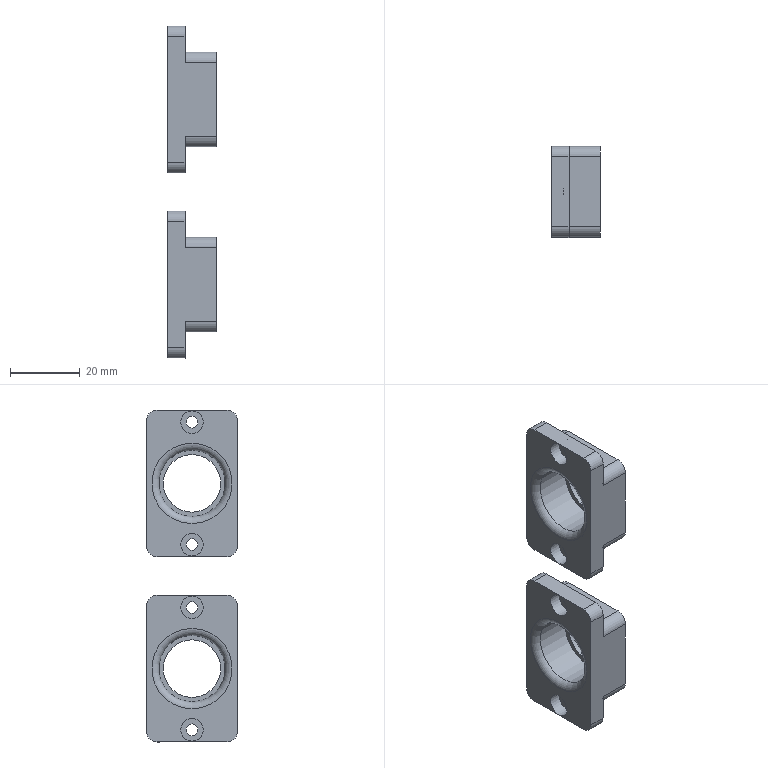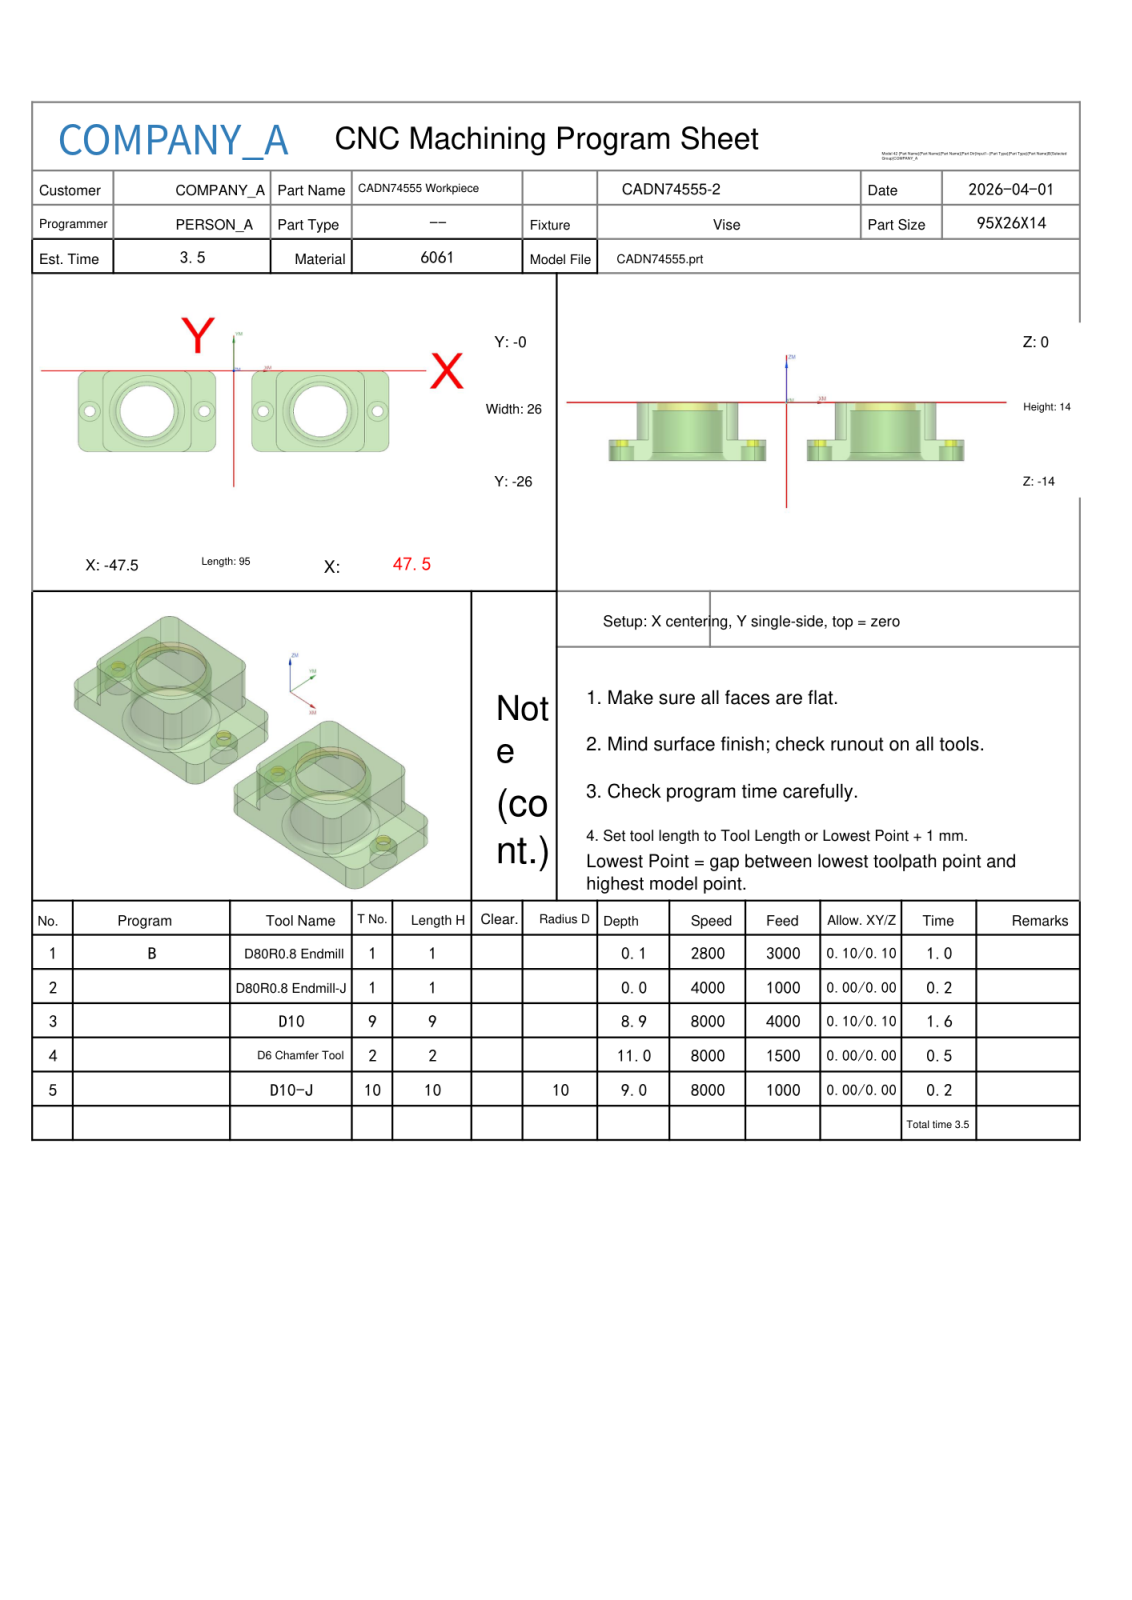NC program | NX | posted by the shop | part box 14 x 26 x 95 mm
Whole program:
%
O0001
(Machine time: 4.41 MIN)
(===Total Tool:4===)
(T1=D80R0.8 Endmill D=80.  R=0.8  D-  H01 Z=0.    )
(T9=D10     D=10.  R=0.   D-  H09 Z=-8.9  )
(T2=D6 Chamfer tool   D=6.   R=0.   D-  H02 Z=-11.  )
(T10=D10-J  D=10.  R=0.   D10 H10 Z=-9.   )
G80 G90 G17 G49 G40
G91 G28 Z0
M01
N1 T01 M06
(D80R0.8 Endmill  D=80. R=0.8 H=01 ce=0.10 di=0.10)
G00 G90 G54 X-99.597 Y-13.002 M03 S2800
G43 H01 Z20.
M08
Z7.009
G01 Z5.009 F3000.
X-87.597
X87.597 Y-12.998
X99.597
Z7.009
G00 X-99.597 Y-13.002
Z6.518
G01 Z4.518
X-87.597
X87.597 Y-12.998
X99.597
Z6.518
G00 X-99.597 Y-13.002
Z6.027
G01 Z4.027
X-87.597
X87.597 Y-12.998
X99.597
Z6.027
G00 X-99.597 Y-13.002
Z5.536
G01 Z3.536
X-87.597
X87.597 Y-12.998
X99.597
Z5.536
G00 Z20.
X-99.597 Y-13.002
Z5.045
G01 Z3.045
X-87.597
X87.597 Y-12.998
X99.597
Z5.045
G00 Z20.
X-99.597 Y-13.002
Z4.555
G01 Z2.555
X-87.597
X87.597 Y-12.998
X99.597
Z4.555
G00 Z20.
X-99.597 Y-13.002
Z4.064
G01 Z2.064
X-87.597
X87.597 Y-12.998
X99.597
Z4.064
G00 Z20.
X-99.597 Y-13.002
Z3.573
G01 Z1.573
X-87.597
X87.597 Y-12.998
X99.597
Z3.573
G00 Z20.
X-99.597 Y-13.002
Z3.082
G01 Z1.082
X-87.597
X87.597 Y-12.998
X99.597
Z3.082
G00 Z20.
X-99.597 Y-13.002
Z2.591
G01 Z.591
X-87.597
X87.597 Y-12.998
X99.597
Z2.591
G00 Z20.
X-99.597 Y-13.002
Z2.1
G01 Z.1
X-87.597
X87.597 Y-12.998
X99.597
Z2.1
G00 Z20.
G91 G28 Z0.0
M05
M09
G91 G28 Z0.0
M01
N2 T01 M06
(D80R0.8 Endmill-J  D=80. R=0.8 H=01 ce=0.00 di=0.00)
G00 G90 G54 X-99.499 Y-13. M03 S4000
G43 H01 Z20.
M08
Z2.
G01 Z0.0 F1000.
X-87.499
X87.499
X99.499
Z2.
G00 Z20.
G91 G28 Z0.0
M05
M09
G91 G28 Z0.0
M01
N3 T09 M06
(D10  D=10. R=0. H=09 ce=0.10 di=0.10)
G00 G90 G54 X-55.5 Y-13. M03 S8000
G43 H09 Z15.5
M08
Z.907
G01 Z-.593 F4000.
X-52.4
Y-3.
G02 X-44.5 Y4.9 I7.9 J0.0
G01 X-38.789
G03 X-45.1 Y-3. I1.789 J-7.9
G01 Y-23.
G03 X-38.789 Y-30.9 I8.1 J0.0
G01 X-44.5
G02 X-52.4 Y-23. I0.0 J7.9
G01 Y-13.
Y-12.5
X-55.5
Z.907
G00 Y-13.
Z.313
G01 Z-1.187
X-52.4
Y-3.
G02 X-44.5 Y4.9 I7.9 J0.0
G01 X-38.789
G03 X-45.1 Y-3. I1.789 J-7.9
G01 Y-23.
G03 X-38.789 Y-30.9 I8.1 J0.0
G01 X-44.5
G02 X-52.4 Y-23. I0.0 J7.9
G01 Y-13.
Y-12.5
X-55.5
Z.313
G00 Y-13.
Z-.28
G01 Z-1.78
X-52.4
Y-3.
G02 X-44.5 Y4.9 I7.9 J0.0
G01 X-38.789
G03 X-45.1 Y-3. I1.789 J-7.9
G01 Y-23.
G03 X-38.789 Y-30.9 I8.1 J0.0
G01 X-44.5
G02 X-52.4 Y-23. I0.0 J7.9
G01 Y-13.
Y-12.5
X-55.5
Z-.28
G00 Y-13.
Z-.873
G01 Z-2.373
X-52.4
Y-3.
G02 X-44.5 Y4.9 I7.9 J0.0
G01 X-38.789
G03 X-45.1 Y-3. I1.789 J-7.9
G01 Y-23.
G03 X-38.789 Y-30.9 I8.1 J0.0
G01 X-44.5
G02 X-52.4 Y-23. I0.0 J7.9
G01 Y-13.
Y-12.5
X-55.5
Z-.873
G00 Y-13.
Z-1.467
G01 Z-2.967
X-52.4
Y-3.
G02 X-44.5 Y4.9 I7.9 J0.0
G01 X-38.789
G03 X-45.1 Y-3. I1.789 J-7.9
G01 Y-23.
G03 X-38.789 Y-30.9 I8.1 J0.0
G01 X-44.5
G02 X-52.4 Y-23. I0.0 J7.9
G01 Y-13.
Y-12.5
X-55.5
Z-1.467
G00 Y-13.
Z-2.06
G01 Z-3.56
X-52.4
Y-3.
G02 X-44.5 Y4.9 I7.9 J0.0
G01 X-38.789
G03 X-45.1 Y-3. I1.789 J-7.9
G01 Y-23.
G03 X-38.789 Y-30.9 I8.1 J0.0
G01 X-44.5
G02 X-52.4 Y-23. I0.0 J7.9
G01 Y-13.
Y-12.5
X-55.5
Z-2.06
G00 Y-13.
Z-2.653
G01 Z-4.153
X-52.4
Y-3.
G02 X-44.5 Y4.9 I7.9 J0.0
G01 X-38.789
G03 X-45.1 Y-3. I1.789 J-7.9
G01 Y-23.
G03 X-38.789 Y-30.9 I8.1 J0.0
G01 X-44.5
G02 X-52.4 Y-23. I0.0 J7.9
G01 Y-13.
Y-12.5
X-55.5
Z-2.653
G00 Y-13.
Z-3.247
G01 Z-4.747
X-52.4
Y-3.
G02 X-44.5 Y4.9 I7.9 J0.0
G01 X-38.789
G03 X-45.1 Y-3. I1.789 J-7.9
G01 Y-23.
G03 X-38.789 Y-30.9 I8.1 J0.0
G01 X-44.5
G02 X-52.4 Y-23. I0.0 J7.9
G01 Y-13.
Y-12.5
X-55.5
Z-3.247
G00 Y-13.
Z-3.84
G01 Z-5.34
X-52.4
Y-3.
G02 X-44.5 Y4.9 I7.9 J0.0
G01 X-38.789
G03 X-45.1 Y-3. I1.789 J-7.9
G01 Y-23.
G03 X-38.789 Y-30.9 I8.1 J0.0
G01 X-44.5
G02 X-52.4 Y-23. I0.0 J7.9
G01 Y-13.
Y-12.5
X-55.5
Z-3.84
G00 Y-13.
Z-4.433
G01 Z-5.933
X-52.4
Y-3.
G02 X-44.5 Y4.9 I7.9 J0.0
G01 X-38.789
G03 X-45.1 Y-3. I1.789 J-7.9
G01 Y-23.
G03 X-38.789 Y-30.9 I8.1 J0.0
G01 X-44.5
G02 X-52.4 Y-23. I0.0 J7.9
G01 Y-13.
Y-12.5
X-55.5
Z-4.433
G00 Y-13.
Z-5.027
G01 Z-6.527
X-52.4
Y-3.
G02 X-44.5 Y4.9 I7.9 J0.0
G01 X-38.789
G03 X-45.1 Y-3. I1.789 J-7.9
G01 Y-23.
G03 X-38.789 Y-30.9 I8.1 J0.0
G01 X-44.5
G02 X-52.4 Y-23. I0.0 J7.9
G01 Y-13.
Y-12.5
X-55.5
Z-5.027
G00 Y-13.
Z-5.62
G01 Z-7.12
X-52.4
Y-3.
G02 X-44.5 Y4.9 I7.9 J0.0
G01 X-38.789
G03 X-45.1 Y-3. I1.789 J-7.9
G01 Y-23.
G03 X-38.789 Y-30.9 I8.1 J0.0
G01 X-44.5
G02 X-52.4 Y-23. I0.0 J7.9
G01 Y-13.
Y-12.5
X-55.5
Z-5.62
G00 Y-13.
Z-6.213
G01 Z-7.713
X-52.4
Y-3.
G02 X-44.5 Y4.9 I7.9 J0.0
G01 X-38.789
G03 X-45.1 Y-3. I1.789 J-7.9
G01 Y-23.
G03 X-38.789 Y-30.9 I8.1 J0.0
G01 X-44.5
G02 X-52.4 Y-23. I0.0 J7.9
G01 Y-13.
Y-12.5
X-55.5
Z-6.213
G00 Y-13.
Z-6.807
G01 Z-8.307
X-52.4
Y-3.
G02 X-44.5 Y4.9 I7.9 J0.0
G01 X-38.789
G03 X-45.1 Y-3. I1.789 J-7.9
G01 Y-23.
G03 X-38.789 Y-30.9 I8.1 J0.0
G01 X-44.5
G02 X-52.4 Y-23. I0.0 J7.9
G01 Y-13.
Y-12.5
X-55.5
Z-6.807
G00 Y-13.
Z-7.4
G01 Z-8.9
X-52.4
Y-3.
G02 X-44.5 Y4.9 I7.9 J0.0
G01 X-38.789
G03 X-45.1 Y-3. I1.789 J-7.9
G01 Y-23.
G03 X-38.789 Y-30.9 I8.1 J0.0
G01 X-44.5
G02 X-52.4 Y-23. I0.0 J7.9
G01 Y-13.
Y-12.5
X-55.5
Z-7.4
G00 Z15.5
X0.0 Y-33.269
Z.907
G01 Z-.593
Y-30.169
X-5.182
X-5.201 Y-30.178
G02 X-8.5 Y-30.9 I-3.299 J7.178
G01 X-14.211
G03 X-7.9 Y-23. I-1.789 J7.9
G01 Y-3.
G03 X-14.211 Y4.9 I-8.1 J0.0
G01 X-8.5
G02 X-5.181 Y4.169 I0.0 J-7.9
G01 X5.201 Y4.178
G02 X8.5 Y4.9 I3.299 J-7.178
G01 X14.211
G03 X7.9 Y-3. I1.789 J-7.9
G01 Y-23.
G03 X14.211 Y-30.9 I8.1 J0.0
G01 X8.5
G02 X5.181 Y-30.169 I0.0 J7.9
G01 X3.222
G02 X2.273 Y-29.486 I0.0 J1.
G01 X.141 Y-23.096
G03 X-.23 Y-22.596 I-.948 J-.317
G02 X-.4 Y-22.271 I.23 J.327
G01 Y-3.729
G02 X0.0 Y-3.331 I.4 J-.001
X.4 Y-3.729 I0.0 J-.4
G01 Y-22.271
G02 X.001 Y-22.669 I-.4 J.001
G01 X-.001
G02 X-.379 Y-22.397 I.001 J.4
G01 X-3.223 Y-23.352
Z.907
G00 X0.0 Y-33.269
Z.313
G01 Z-1.187
Y-30.169
X-5.182
X-5.201 Y-30.178
G02 X-8.5 Y-30.9 I-3.299 J7.178
G01 X-14.211
G03 X-7.9 Y-23. I-1.789 J7.9
G01 Y-3.
G03 X-14.211 Y4.9 I-8.1 J0.0
G01 X-8.5
G02 X-5.181 Y4.169 I0.0 J-7.9
G01 X5.201 Y4.178
G02 X8.5 Y4.9 I3.299 J-7.178
G01 X14.211
G03 X7.9 Y-3. I1.789 J-7.9
G01 Y-23.
G03 X14.211 Y-30.9 I8.1 J0.0
G01 X8.5
G02 X5.181 Y-30.169 I0.0 J7.9
G01 X3.222
G02 X2.273 Y-29.486 I0.0 J1.
G01 X.141 Y-23.096
G03 X-.23 Y-22.596 I-.948 J-.317
G02 X-.4 Y-22.271 I.23 J.327
G01 Y-3.729
G02 X0.0 Y-3.331 I.4 J-.001
X.4 Y-3.729 I0.0 J-.4
G01 Y-22.271
G02 X.001 Y-22.669 I-.4 J.001
G01 X-.001
G02 X-.379 Y-22.397 I.001 J.4
G01 X-3.223 Y-23.352
Z.313
G00 X0.0 Y-33.269
Z-.28
G01 Z-1.78
Y-30.169
X-5.182
X-5.201 Y-30.178
G02 X-8.5 Y-30.9 I-3.299 J7.178
G01 X-14.211
G03 X-7.9 Y-23. I-1.789 J7.9
G01 Y-3.
G03 X-14.211 Y4.9 I-8.1 J0.0
G01 X-8.5
G02 X-5.181 Y4.169 I0.0 J-7.9
G01 X5.201 Y4.178
G02 X8.5 Y4.9 I3.299 J-7.178
G01 X14.211
G03 X7.9 Y-3. I1.789 J-7.9
G01 Y-23.
G03 X14.211 Y-30.9 I8.1 J0.0
G01 X8.5
G02 X5.181 Y-30.169 I0.0 J7.9
G01 X3.222
G02 X2.273 Y-29.486 I0.0 J1.
G01 X.141 Y-23.096
G03 X-.23 Y-22.596 I-.948 J-.317
G02 X-.4 Y-22.271 I.23 J.327
G01 Y-3.729
G02 X0.0 Y-3.331 I.4 J-.001
X.4 Y-3.729 I0.0 J-.4
G01 Y-22.271
G02 X.001 Y-22.669 I-.4 J.001
G01 X-.001
G02 X-.379 Y-22.397 I.001 J.4
G01 X-3.223 Y-23.352
Z-.28
G00 X0.0 Y-33.269
Z-.873
G01 Z-2.373
Y-30.169
X-5.182
X-5.201 Y-30.178
G02 X-8.5 Y-30.9 I-3.299 J7.178
G01 X-14.211
G03 X-7.9 Y-23. I-1.789 J7.9
G01 Y-3.
G03 X-14.211 Y4.9 I-8.1 J0.0
G01 X-8.5
G02 X-5.181 Y4.169 I0.0 J-7.9
G01 X5.201 Y4.178
G02 X8.5 Y4.9 I3.299 J-7.178
G01 X14.211
G03 X7.9 Y-3. I1.789 J-7.9
G01 Y-23.
G03 X14.211 Y-30.9 I8.1 J0.0
G01 X8.5
G02 X5.181 Y-30.169 I0.0 J7.9
G01 X3.222
G02 X2.273 Y-29.486 I0.0 J1.
G01 X.141 Y-23.096
G03 X-.23 Y-22.596 I-.948 J-.317
G02 X-.4 Y-22.271 I.23 J.327
G01 Y-3.729
G02 X0.0 Y-3.331 I.4 J-.001
X.4 Y-3.729 I0.0 J-.4
G01 Y-22.271
G02 X.001 Y-22.669 I-.4 J.001
G01 X-.001
G02 X-.379 Y-22.397 I.001 J.4
G01 X-3.223 Y-23.352
Z-.873
G00 X0.0 Y-33.269
Z-1.467
G01 Z-2.967
Y-30.169
X-5.182
X-5.201 Y-30.178
G02 X-8.5 Y-30.9 I-3.299 J7.178
G01 X-14.211
G03 X-7.9 Y-23. I-1.789 J7.9
G01 Y-3.
G03 X-14.211 Y4.9 I-8.1 J0.0
G01 X-8.5
G02 X-5.181 Y4.169 I0.0 J-7.9
G01 X5.201 Y4.178
G02 X8.5 Y4.9 I3.299 J-7.178
G01 X14.211
G03 X7.9 Y-3. I1.789 J-7.9
G01 Y-23.
G03 X14.211 Y-30.9 I8.1 J0.0
G01 X8.5
G02 X5.181 Y-30.169 I0.0 J7.9
G01 X3.222
G02 X2.273 Y-29.486 I0.0 J1.
G01 X.141 Y-23.096
G03 X-.23 Y-22.596 I-.948 J-.317
G02 X-.4 Y-22.271 I.23 J.327
G01 Y-3.729
G02 X0.0 Y-3.331 I.4 J-.001
X.4 Y-3.729 I0.0 J-.4
G01 Y-22.271
G02 X.001 Y-22.669 I-.4 J.001
G01 X-.001
G02 X-.379 Y-22.397 I.001 J.4
G01 X-3.223 Y-23.352
Z-1.467
G00 X0.0 Y-33.269
Z-2.06
G01 Z-3.56
Y-30.169
X-5.182
X-5.201 Y-30.178
G02 X-8.5 Y-30.9 I-3.299 J7.178
G01 X-14.211
G03 X-7.9 Y-23. I-1.789 J7.9
G01 Y-3.
G03 X-14.211 Y4.9 I-8.1 J0.0
G01 X-8.5
G02 X-5.181 Y4.169 I0.0 J-7.9
G01 X5.201 Y4.178
G02 X8.5 Y4.9 I3.299 J-7.178
G01 X14.211
G03 X7.9 Y-3. I1.789 J-7.9
G01 Y-23.
G03 X14.211 Y-30.9 I8.1 J0.0
G01 X8.5
G02 X5.181 Y-30.169 I0.0 J7.9
G01 X3.222
G02 X2.273 Y-29.486 I0.0 J1.
G01 X.141 Y-23.096
G03 X-.23 Y-22.596 I-.948 J-.317
G02 X-.4 Y-22.271 I.23 J.327
G01 Y-3.729
G02 X0.0 Y-3.331 I.4 J-.001
X.4 Y-3.729 I0.0 J-.4
G01 Y-22.271
G02 X.001 Y-22.669 I-.4 J.001
G01 X-.001
G02 X-.379 Y-22.397 I.001 J.4
G01 X-3.223 Y-23.352
Z-2.06
G00 X0.0 Y-33.269
Z-2.653
G01 Z-4.153
Y-30.169
X-5.182
X-5.201 Y-30.178
G02 X-8.5 Y-30.9 I-3.299 J7.178
G01 X-14.211
G03 X-7.9 Y-23. I-1.789 J7.9
G01 Y-3.
G03 X-14.211 Y4.9 I-8.1 J0.0
G01 X-8.5
G02 X-5.181 Y4.169 I0.0 J-7.9
G01 X5.201 Y4.178
G02 X8.5 Y4.9 I3.299 J-7.178
G01 X14.211
G03 X7.9 Y-3. I1.789 J-7.9
G01 Y-23.
G03 X14.211 Y-30.9 I8.1 J0.0
G01 X8.5
G02 X5.181 Y-30.169 I0.0 J7.9
G01 X3.222
G02 X2.273 Y-29.486 I0.0 J1.
G01 X.141 Y-23.096
G03 X-.23 Y-22.596 I-.948 J-.317
G02 X-.4 Y-22.271 I.23 J.327
G01 Y-3.729
G02 X0.0 Y-3.331 I.4 J-.001
X.4 Y-3.729 I0.0 J-.4
G01 Y-22.271
G02 X.001 Y-22.669 I-.4 J.001
G01 X-.001
G02 X-.379 Y-22.397 I.001 J.4
G01 X-3.223 Y-23.352
Z-2.653
G00 X0.0 Y-33.269
Z-3.247
G01 Z-4.747
Y-30.169
X-5.182
X-5.201 Y-30.178
G02 X-8.5 Y-30.9 I-3.299 J7.178
G01 X-14.211
G03 X-7.9 Y-23. I-1.789 J7.9
G01 Y-3.
G03 X-14.211 Y4.9 I-8.1 J0.0
G01 X-8.5
G02 X-5.181 Y4.169 I0.0 J-7.9
G01 X5.201 Y4.178
G02 X8.5 Y4.9 I3.299 J-7.178
G01 X14.211
G03 X7.9 Y-3. I1.789 J-7.9
G01 Y-23.
G03 X14.211 Y-30.9 I8.1 J0.0
G01 X8.5
G02 X5.181 Y-30.169 I0.0 J7.9
G01 X3.222
G02 X2.273 Y-29.486 I0.0 J1.
G01 X.141 Y-23.096
G03 X-.23 Y-22.596 I-.948 J-.317
G02 X-.4 Y-22.271 I.23 J.327
G01 Y-3.729
G02 X0.0 Y-3.331 I.4 J-.001
X.4 Y-3.729 I0.0 J-.4
G01 Y-22.271
G02 X.001 Y-22.669 I-.4 J.001
G01 X-.001
G02 X-.379 Y-22.397 I.001 J.4
G01 X-3.223 Y-23.352
Z-3.247
G00 X0.0 Y-33.269
Z-3.84
G01 Z-5.34
Y-30.169
X-5.182
X-5.201 Y-30.178
G02 X-8.5 Y-30.9 I-3.299 J7.178
G01 X-14.211
G03 X-7.9 Y-23. I-1.789 J7.9
G01 Y-3.
G03 X-14.211 Y4.9 I-8.1 J0.0
G01 X-8.5
G02 X-5.181 Y4.169 I0.0 J-7.9
G01 X5.201 Y4.178
G02 X8.5 Y4.9 I3.299 J-7.178
G01 X14.211
G03 X7.9 Y-3. I1.789 J-7.9
G01 Y-23.
G03 X14.211 Y-30.9 I8.1 J0.0
G01 X8.5
G02 X5.181 Y-30.169 I0.0 J7.9
G01 X3.222
G02 X2.273 Y-29.486 I0.0 J1.
G01 X.141 Y-23.096
G03 X-.23 Y-22.596 I-.948 J-.317
G02 X-.4 Y-22.271 I.23 J.327
G01 Y-3.729
G02 X0.0 Y-3.331 I.4 J-.001
X.4 Y-3.729 I0.0 J-.4
G01 Y-22.271
G02 X.001 Y-22.669 I-.4 J.001
G01 X-.001
G02 X-.379 Y-22.397 I.001 J.4
G01 X-3.223 Y-23.352
Z-3.84
G00 X0.0 Y-33.269
Z-4.433
G01 Z-5.933
Y-30.169
X-5.182
X-5.201 Y-30.178
G02 X-8.5 Y-30.9 I-3.299 J7.178
G01 X-14.211
G03 X-7.9 Y-23. I-1.789 J7.9
G01 Y-3.
G03 X-14.211 Y4.9 I-8.1 J0.0
G01 X-8.5
G02 X-5.181 Y4.169 I0.0 J-7.9
G01 X5.201 Y4.178
G02 X8.5 Y4.9 I3.299 J-7.178
G01 X14.211
G03 X7.9 Y-3. I1.789 J-7.9
G01 Y-23.
G03 X14.211 Y-30.9 I8.1 J0.0
G01 X8.5
G02 X5.181 Y-30.169 I0.0 J7.9
G01 X3.222
G02 X2.273 Y-29.486 I0.0 J1.
G01 X.141 Y-23.096
G03 X-.23 Y-22.596 I-.948 J-.317
G02 X-.4 Y-22.271 I.23 J.327
G01 Y-3.729
G02 X0.0 Y-3.331 I.4 J-.001
X.4 Y-3.729 I0.0 J-.4
G01 Y-22.271
G02 X.001 Y-22.669 I-.4 J.001
G01 X-.001
G02 X-.379 Y-22.397 I.001 J.4
G01 X-3.223 Y-23.352
Z-4.433
G00 X0.0 Y-33.269
Z-5.027
G01 Z-6.527
Y-30.169
X-5.182
X-5.201 Y-30.178
G02 X-8.5 Y-30.9 I-3.299 J7.178
G01 X-14.211
G03 X-7.9 Y-23. I-1.789 J7.9
G01 Y-3.
G03 X-14.211 Y4.9 I-8.1 J0.0
G01 X-8.5
G02 X-5.181 Y4.169 I0.0 J-7.9
G01 X5.201 Y4.178
G02 X8.5 Y4.9 I3.299 J-7.178
G01 X14.211
G03 X7.9 Y-3. I1.789 J-7.9
G01 Y-23.
G03 X14.211 Y-30.9 I8.1 J0.0
G01 X8.5
G02 X5.181 Y-30.169 I0.0 J7.9
G01 X3.222
G02 X2.273 Y-29.486 I0.0 J1.
G01 X.141 Y-23.096
G03 X-.23 Y-22.596 I-.948 J-.317
G02 X-.4 Y-22.271 I.23 J.327
G01 Y-3.729
G02 X0.0 Y-3.331 I.4 J-.001
X.4 Y-3.729 I0.0 J-.4
G01 Y-22.271
G02 X.001 Y-22.669 I-.4 J.001
G01 X-.001
G02 X-.379 Y-22.397 I.001 J.4
G01 X-3.223 Y-23.352
Z-5.027
G00 X0.0 Y-33.269
Z-5.62
G01 Z-7.12
Y-30.169
X-5.182
X-5.201 Y-30.178
G02 X-8.5 Y-30.9 I-3.299 J7.178
G01 X-14.211
G03 X-7.9 Y-23. I-1.789 J7.9
G01 Y-3.
G03 X-14.211 Y4.9 I-8.1 J0.0
G01 X-8.5
G02 X-5.181 Y4.169 I0.0 J-7.9
G01 X5.201 Y4.178
G02 X8.5 Y4.9 I3.299 J-7.178
G01 X14.211
G03 X7.9 Y-3. I1.789 J-7.9
G01 Y-23.
G03 X14.211 Y-30.9 I8.1 J0.0
G01 X8.5
G02 X5.181 Y-30.169 I0.0 J7.9
G01 X3.222
G02 X2.273 Y-29.486 I0.0 J1.
G01 X.141 Y-23.096
G03 X-.23 Y-22.596 I-.948 J-.317
G02 X-.4 Y-22.271 I.23 J.327
G01 Y-3.729
G02 X0.0 Y-3.331 I.4 J-.001
X.4 Y-3.729 I0.0 J-.4
G01 Y-22.271
G02 X.001 Y-22.669 I-.4 J.001
G01 X-.001
G02 X-.379 Y-22.397 I.001 J.4
G01 X-3.223 Y-23.352
Z-5.62
G00 X0.0 Y-33.269
Z-6.213
G01 Z-7.713
Y-30.169
X-5.182
X-5.201 Y-30.178
G02 X-8.5 Y-30.9 I-3.299 J7.178
G01 X-14.211
G03 X-7.9 Y-23. I-1.789 J7.9
G01 Y-3.
G03 X-14.211 Y4.9 I-8.1 J0.0
G01 X-8.5
G02 X-5.181 Y4.169 I0.0 J-7.9
G01 X5.201 Y4.178
G02 X8.5 Y4.9 I3.299 J-7.178
G01 X14.211
G03 X7.9 Y-3. I1.789 J-7.9
G01 Y-23.
G03 X14.211 Y-30.9 I8.1 J0.0
G01 X8.5
G02 X5.181 Y-30.169 I0.0 J7.9
G01 X3.222
G02 X2.273 Y-29.486 I0.0 J1.
G01 X.141 Y-23.096
G03 X-.23 Y-22.596 I-.948 J-.317
G02 X-.4 Y-22.271 I.23 J.327
G01 Y-3.729
G02 X0.0 Y-3.331 I.4 J-.001
X.4 Y-3.729 I0.0 J-.4
G01 Y-22.271
G02 X.001 Y-22.669 I-.4 J.001
G01 X-.001
G02 X-.379 Y-22.397 I.001 J.4
G01 X-3.223 Y-23.352
Z-6.213
G00 X0.0 Y-33.269
Z-6.807
G01 Z-8.307
Y-30.169
X-5.182
X-5.201 Y-30.178
G02 X-8.5 Y-30.9 I-3.299 J7.178
G01 X-14.211
G03 X-7.9 Y-23. I-1.789 J7.9
G01 Y-3.
G03 X-14.211 Y4.9 I-8.1 J0.0
G01 X-8.5
G02 X-5.181 Y4.169 I0.0 J-7.9
G01 X5.201 Y4.178
G02 X8.5 Y4.9 I3.299 J-7.178
G01 X14.211
G03 X7.9 Y-3. I1.789 J-7.9
G01 Y-23.
G03 X14.211 Y-30.9 I8.1 J0.0
G01 X8.5
G02 X5.181 Y-30.169 I0.0 J7.9
G01 X3.222
G02 X2.273 Y-29.486 I0.0 J1.
G01 X.141 Y-23.096
G03 X-.23 Y-22.596 I-.948 J-.317
G02 X-.4 Y-22.271 I.23 J.327
G01 Y-3.729
G02 X0.0 Y-3.331 I.4 J-.001
X.4 Y-3.729 I0.0 J-.4
G01 Y-22.271
G02 X.001 Y-22.669 I-.4 J.001
G01 X-.001
G02 X-.379 Y-22.397 I.001 J.4
G01 X-3.223 Y-23.352
Z-6.807
G00 X0.0 Y-33.269
Z-7.4
G01 Z-8.9
Y-30.169
X-5.182
X-5.201 Y-30.178
G02 X-8.5 Y-30.9 I-3.299 J7.178
G01 X-14.211
G03 X-7.9 Y-23. I-1.789 J7.9
G01 Y-3.
G03 X-14.211 Y4.9 I-8.1 J0.0
G01 X-8.5
G02 X-5.181 Y4.169 I0.0 J-7.9
G01 X5.201 Y4.178
G02 X8.5 Y4.9 I3.299 J-7.178
G01 X14.211
G03 X7.9 Y-3. I1.789 J-7.9
G01 Y-23.
G03 X14.211 Y-30.9 I8.1 J0.0
G01 X8.5
G02 X5.181 Y-30.169 I0.0 J7.9
G01 X3.222
G02 X2.273 Y-29.486 I0.0 J1.
G01 X.141 Y-23.096
G03 X-.23 Y-22.596 I-.948 J-.317
G02 X-.4 Y-22.271 I.23 J.327
G01 Y-3.729
G02 X0.0 Y-3.331 I.4 J-.001
X.4 Y-3.729 I0.0 J-.4
G01 Y-22.271
G02 X.001 Y-22.669 I-.4 J.001
G01 X-.001
G02 X-.379 Y-22.397 I.001 J.4
G01 X-3.223 Y-23.352
Z-7.4
G00 Z15.5
X55.5 Y-13.
Z.907
G01 Z-.593
X52.4
Y-23.
G02 X44.5 Y-30.9 I-7.9 J0.0
G01 X38.789
G03 X45.1 Y-23. I-1.789 J7.9
G01 Y-3.
G03 X38.789 Y4.9 I-8.1 J0.0
G01 X44.5
G02 X52.4 Y-3. I0.0 J-7.9
G01 Y-13.
Y-13.5
X55.5
Z.907
G00 Y-13.
Z.313
G01 Z-1.187
X52.4
Y-23.
G02 X44.5 Y-30.9 I-7.9 J0.0
G01 X38.789
G03 X45.1 Y-23. I-1.789 J7.9
G01 Y-3.
G03 X38.789 Y4.9 I-8.1 J0.0
G01 X44.5
G02 X52.4 Y-3. I0.0 J-7.9
G01 Y-13.
Y-13.5
X55.5
Z.313
G00 Y-13.
Z-.28
G01 Z-1.78
X52.4
Y-23.
G02 X44.5 Y-30.9 I-7.9 J0.0
G01 X38.789
G03 X45.1 Y-23. I-1.789 J7.9
G01 Y-3.
G03 X38.789 Y4.9 I-8.1 J0.0
G01 X44.5
G02 X52.4 Y-3. I0.0 J-7.9
G01 Y-13.
Y-13.5
X55.5
Z-.28
G00 Y-13.
Z-.873
G01 Z-2.373
X52.4
Y-23.
G02 X44.5 Y-30.9 I-7.9 J0.0
G01 X38.789
G03 X45.1 Y-23. I-1.789 J7.9
G01 Y-3.
G03 X38.789 Y4.9 I-8.1 J0.0
G01 X44.5
G02 X52.4 Y-3. I0.0 J-7.9
G01 Y-13.
Y-13.5
X55.5
Z-.873
G00 Y-13.
Z-1.467
G01 Z-2.967
X52.4
Y-23.
G02 X44.5 Y-30.9 I-7.9 J0.0
G01 X38.789
G03 X45.1 Y-23. I-1.789 J7.9
G01 Y-3.
G03 X38.789 Y4.9 I-8.1 J0.0
G01 X44.5
G02 X52.4 Y-3. I0.0 J-7.9
G01 Y-13.
Y-13.5
X55.5
Z-1.467
G00 Y-13.
Z-2.06
G01 Z-3.56
X52.4
Y-23.
G02 X44.5 Y-30.9 I-7.9 J0.0
G01 X38.789
G03 X45.1 Y-23. I-1.789 J7.9
G01 Y-3.
G03 X38.789 Y4.9 I-8.1 J0.0
G01 X44.5
G02 X52.4 Y-3. I0.0 J-7.9
G01 Y-13.
Y-13.5
X55.5
Z-2.06
G00 Y-13.
Z-2.653
G01 Z-4.153
X52.4
Y-23.
G02 X44.5 Y-30.9 I-7.9 J0.0
G01 X38.789
G03 X45.1 Y-23. I-1.789 J7.9
G01 Y-3.
G03 X38.789 Y4.9 I-8.1 J0.0
G01 X44.5
G02 X52.4 Y-3. I0.0 J-7.9
G01 Y-13.
Y-13.5
X55.5
Z-2.653
G00 Y-13.
Z-3.247
G01 Z-4.747
X52.4
Y-23.
G02 X44.5 Y-30.9 I-7.9 J0.0
G01 X38.789
G03 X45.1 Y-23. I-1.789 J7.9
G01 Y-3.
G03 X38.789 Y4.9 I-8.1 J0.0
G01 X44.5
G02 X52.4 Y-3. I0.0 J-7.9
G01 Y-13.
Y-13.5
X55.5
Z-3.247
G00 Y-13.
Z-3.84
G01 Z-5.34
X52.4
Y-23.
G02 X44.5 Y-30.9 I-7.9 J0.0
G01 X38.789
G03 X45.1 Y-23. I-1.789 J7.9
G01 Y-3.
G03 X38.789 Y4.9 I-8.1 J0.0
G01 X44.5
G02 X52.4 Y-3. I0.0 J-7.9
G01 Y-13.
Y-13.5
X55.5
Z-3.84
G00 Y-13.
Z-4.433
G01 Z-5.933
X52.4
Y-23.
G02 X44.5 Y-30.9 I-7.9 J0.0
G01 X38.789
G03 X45.1 Y-23. I-1.789 J7.9
G01 Y-3.
G03 X38.789 Y4.9 I-8.1 J0.0
G01 X44.5
G02 X52.4 Y-3. I0.0 J-7.9
G01 Y-13.
Y-13.5
X55.5
Z-4.433
G00 Y-13.
Z-5.027
G01 Z-6.527
X52.4
Y-23.
G02 X44.5 Y-30.9 I-7.9 J0.0
G01 X38.789
G03 X45.1 Y-23. I-1.789 J7.9
G01 Y-3.
G03 X38.789 Y4.9 I-8.1 J0.0
G01 X44.5
G02 X52.4 Y-3. I0.0 J-7.9
G01 Y-13.
Y-13.5
X55.5
Z-5.027
G00 Y-13.
Z-5.62
G01 Z-7.12
X52.4
Y-23.
G02 X44.5 Y-30.9 I-7.9 J0.0
G01 X38.789
G03 X45.1 Y-23. I-1.789 J7.9
G01 Y-3.
G03 X38.789 Y4.9 I-8.1 J0.0
G01 X44.5
G02 X52.4 Y-3. I0.0 J-7.9
G01 Y-13.
Y-13.5
X55.5
Z-5.62
G00 Y-13.
Z-6.213
G01 Z-7.713
X52.4
Y-23.
G02 X44.5 Y-30.9 I-7.9 J0.0
G01 X38.789
G03 X45.1 Y-23. I-1.789 J7.9
G01 Y-3.
G03 X38.789 Y4.9 I-8.1 J0.0
G01 X44.5
G02 X52.4 Y-3. I0.0 J-7.9
G01 Y-13.
Y-13.5
X55.5
Z-6.213
G00 Y-13.
Z-6.807
G01 Z-8.307
X52.4
Y-23.
G02 X44.5 Y-30.9 I-7.9 J0.0
G01 X38.789
G03 X45.1 Y-23. I-1.789 J7.9
G01 Y-3.
G03 X38.789 Y4.9 I-8.1 J0.0
G01 X44.5
G02 X52.4 Y-3. I0.0 J-7.9
G01 Y-13.
Y-13.5
X55.5
Z-6.807
G00 Y-13.
Z-7.4
G01 Z-8.9
X52.4
Y-23.
G02 X44.5 Y-30.9 I-7.9 J0.0
G01 X38.789
G03 X45.1 Y-23. I-1.789 J7.9
G01 Y-3.
G03 X38.789 Y4.9 I-8.1 J0.0
G01 X44.5
G02 X52.4 Y-3. I0.0 J-7.9
G01 Y-13.
Y-13.5
X55.5
Z-7.4
G00 Z15.5
G91 G28 Z0.0
M05
M09
G91 G28 Z0.0
M01
N4 T02 M06
(D6 Chamfer tool  D=6. R=0. H=02 ce=0.00 di=0.10)
G00 G90 G54 X-44. Y-13. M03 S8000
G43 H02 Z20.
M08
G98 G81 X-44. Y-13. Z-11. R-6. F1000.
X-9.
X9.
X44.
G80
G00 Z20.
G00 G90 X-26.886 Y.827 M03 S6500
Z20.
Z.572
G01 Z-.799 F1500.
G03 X-26.6 Y.627 I1.286 J1.532
G01 X-26.554 Y.597
X-26.5 Y.6
X-16.
G02 X-12.4 Y-3. I0.0 J-3.6
G01 Y-23.
G02 X-16. Y-26.6 I-3.6 J0.0
G01 X-37.
G02 X-40.6 Y-23. I0.0 J3.6
G01 Y-3.
G02 X-37. Y.6 I3.6 J0.0
G01 X-26.5
X-26.446 Y.597
X-26.4 Y.627
G03 X-26.114 Y.827 I-1. J1.732
G01 Z.572
G00 Z10.
X-19.058 Y-13.396
Z.602
G01 Z-.799
G03 X-18.872 Y-13.101 I-1.592 J1.211
G01 X-18.845 Y-13.054
X-18.85 Y-13.
G03 X-26.5 Y-5.35 I-7.65 J0.0
X-34.15 Y-13. I0.0 J-7.65
X-26.5 Y-20.65 I7.65 J0.0
X-18.85 Y-13. I0.0 J7.65
G01 X-18.845 Y-12.946
X-18.872 Y-12.899
G03 X-19.058 Y-12.604 I-1.778 J-.916
G01 Z.602
G00 Z10.
X12.173 Y-13.386
Z.572
G01 Z-.799
G03 X12.373 Y-13.1 I-1.532 J1.286
G01 X12.403 Y-13.054
X12.4 Y-13.
Y-3.
G02 X16. Y.6 I3.6 J0.0
G01 X37.
G02 X40.6 Y-3. I0.0 J-3.6
G01 Y-23.
G02 X37. Y-26.6 I-3.6 J0.0
G01 X16.
G02 X12.4 Y-23. I0.0 J3.6
G01 Y-13.
X12.403 Y-12.946
X12.373 Y-12.9
G03 X12.173 Y-12.614 I-1.732 J-1.
G01 Z.572
G00 Z10.
X33.942 Y-13.396
Z.602
G01 Z-.799
G03 X34.128 Y-13.101 I-1.592 J1.211
G01 X34.155 Y-13.054
X34.15 Y-13.
G03 X26.5 Y-5.35 I-7.65 J0.0
X18.85 Y-13. I0.0 J-7.65
X26.5 Y-20.65 I7.65 J0.0
X34.15 Y-13. I0.0 J7.65
G01 X34.155 Y-12.946
X34.128 Y-12.899
G03 X33.942 Y-12.604 I-1.778 J-.916
G01 Z.602
G00 Z10.
X41.963 Y.713
Z-1.801
G01 Z-9.799
X42.027 Y.652
X42.106 Y.613
X42.128 Y.594
X42.156 Y.6
X44.5
G02 X48.1 Y-3. I0.0 J-3.6
G01 Y-23.
G02 X44.5 Y-26.6 I-3.6 J0.0
G01 X42.156
X42.128 Y-26.594
X42.106 Y-26.613
X42.027 Y-26.652
X41.963 Y-26.713
Z-1.801
G00 Z10.
X43.195 Y-13.614
Z-1.797
G01 Z-9.799
X43.208 Y-13.701
X43.248 Y-13.78
X43.253 Y-13.809
X43.279 Y-13.822
X43.45 Y-13.953
G03 X44. Y-14.1 I.55 J.953
X45.1 Y-13. I0.0 J1.1
X44. Y-11.9 I-1.1 J0.0
X43.45 Y-12.047 I0.0 J-1.1
G01 X43.279 Y-12.178
X43.253 Y-12.191
X43.248 Y-12.22
X43.208 Y-12.299
X43.195 Y-12.386
Z-1.797
G00 Z10.
X11.037 Y-26.713
Z-1.801
G01 Z-9.799
X10.973 Y-26.652
X10.894 Y-26.613
X10.872 Y-26.594
X10.844 Y-26.6
X8.5
G02 X4.9 Y-23. I0.0 J3.6
G01 Y-3.
G02 X8.5 Y.6 I3.6 J0.0
G01 X10.844
X10.872 Y.594
X10.894 Y.613
X10.973 Y.652
X11.037 Y.713
Z-1.801
G00 Z10.
X9.805 Y-12.386
Z-1.797
G01 Z-9.799
X9.792 Y-12.299
X9.752 Y-12.22
X9.747 Y-12.191
X9.721 Y-12.178
X9.55 Y-12.047
G03 X9. Y-11.9 I-.55 J-.953
X7.9 Y-13. I0.0 J-1.1
X9. Y-14.1 I1.1 J0.0
X9.55 Y-13.953 I0.0 J1.1
G01 X9.721 Y-13.822
X9.747 Y-13.809
X9.752 Y-13.78
X9.792 Y-13.701
X9.805 Y-13.614
Z-1.797
G00 Z10.
X-11.037 Y.713
Z-1.801
G01 Z-9.799
X-10.973 Y.652
X-10.894 Y.613
X-10.872 Y.594
X-10.844 Y.6
X-8.5
G02 X-4.9 Y-3. I0.0 J-3.6
G01 Y-23.
G02 X-8.5 Y-26.6 I-3.6 J0.0
G01 X-10.844
X-10.872 Y-26.594
X-10.894 Y-26.613
X-10.973 Y-26.652
X-11.037 Y-26.713
Z-1.801
G00 Z10.
X-9.805 Y-13.614
Z-1.797
G01 Z-9.799
X-9.792 Y-13.701
X-9.752 Y-13.78
X-9.747 Y-13.809
X-9.721 Y-13.822
X-9.55 Y-13.953
G03 X-9. Y-14.1 I.55 J.953
X-7.9 Y-13. I0.0 J1.1
X-9. Y-11.9 I-1.1 J0.0
X-9.55 Y-12.047 I0.0 J-1.1
G01 X-9.721 Y-12.178
X-9.747 Y-12.191
X-9.752 Y-12.22
X-9.792 Y-12.299
X-9.805 Y-12.386
Z-1.797
G00 Z10.
X-41.963 Y-26.713
Z-1.801
G01 Z-9.799
X-42.027 Y-26.652
X-42.106 Y-26.613
X-42.128 Y-26.594
X-42.156 Y-26.6
X-44.5
G02 X-48.1 Y-23. I0.0 J3.6
G01 Y-3.
G02 X-44.5 Y.6 I3.6 J0.0
G01 X-42.156
X-42.128 Y.594
X-42.106 Y.613
X-42.027 Y.652
X-41.963 Y.713
Z-1.801
G00 Z10.
X-43.195 Y-12.386
Z-1.797
G01 Z-9.799
X-43.208 Y-12.299
X-43.248 Y-12.22
X-43.253 Y-12.191
X-43.279 Y-12.178
X-43.45 Y-12.047
G03 X-44. Y-11.9 I-.55 J-.953
X-45.1 Y-13. I0.0 J-1.1
X-44. Y-14.1 I1.1 J0.0
X-43.45 Y-13.953 I0.0 J1.1
G01 X-43.279 Y-13.822
X-43.253 Y-13.809
X-43.248 Y-13.78
X-43.208 Y-13.701
X-43.195 Y-13.614
Z-1.797
G00 Z20.
G91 G28 Z0.0
M05
M09
G91 G28 Z0.0
M01
N5 T10 M06
(D10-J  D=10. R=0. H=10 ce=0.00 di=0.00)
G00 G90 G54 X-35.274 Y-33.2 M03 S8000
G43 H10 Z15.5
M08
Z-8.
G01 Z-9. F1000.
G41 D10
Y-33.
Y-32.996
G03 X-37.219 Y-30.997 I-2. J0.0
G02 X-45. Y-23. I.219 J7.997
G01 Y-3.
G02 X-37.219 Y4.997 I8. J0.0
G03 X-35.274 Y6.996 I-.055 J1.999
G01 Y7.
G40 Y7.2
Z-8.
G00 Z3.
X-17.726
Z-8.
G01 Z-9.
G41 D10
Y7.
Y6.996
G03 X-15.781 Y4.997 I2. J0.0
G02 X-8. Y-3. I-.219 J-7.997
G01 Y-23.
G02 X-15.781 Y-30.997 I-8. J0.0
G03 X-17.726 Y-32.996 I.055 J-1.999
G01 Y-33.
G40 Y-33.2
Z-8.
G00 X17.726
G01 Z-9.
G41 D10
Y-33.
Y-32.996
G03 X15.781 Y-30.997 I-2. J0.0
G02 X8. Y-23. I.219 J7.997
G01 Y-3.
G02 X15.781 Y4.997 I8. J0.0
G03 X17.726 Y6.996 I-.055 J1.999
G01 Y7.
G40 Y7.2
Z-8.
G00 Z3.
X35.274
Z-8.
G01 Z-9.
G41 D10
Y7.
Y6.996
G03 X37.219 Y4.997 I2. J0.0
G02 X45. Y-3. I-.219 J-7.997
G01 Y-23.
G02 X37.219 Y-30.997 I-8. J0.0
G03 X35.274 Y-32.996 I.055 J-1.999
G01 Y-33.
G40 Y-33.2
Z-8.
G00 Z15.5
M05
M09
G91 G28 Z0.0
G91 G28 Y0.0
M30
%